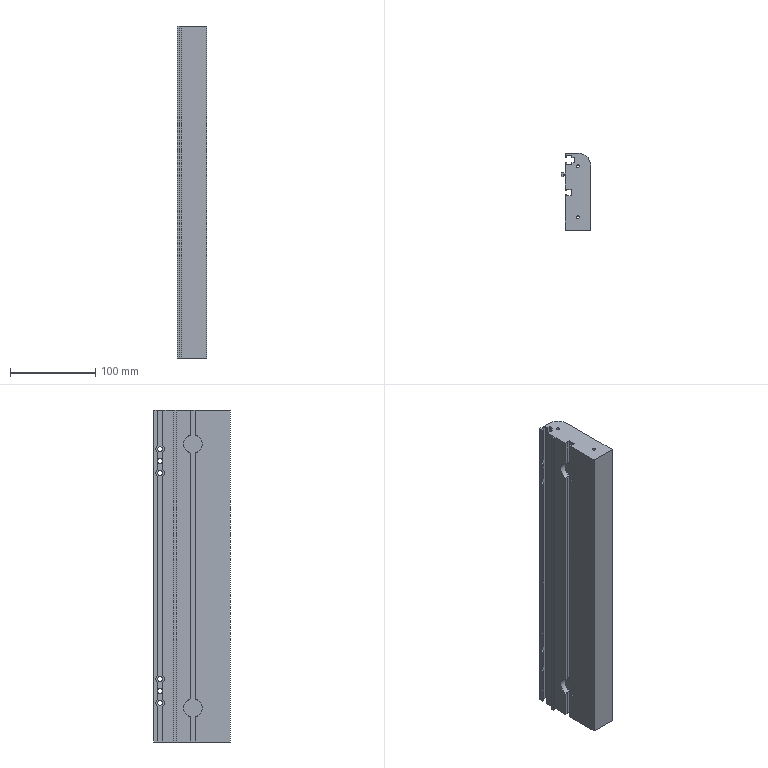Part | SolidWorks | features ICE 3, HoleWzd 2, MirrorPattern 2, Extrusion 1 | 1 solid | 115 faces | box 34.5 x 90 x 390 mm | volume 934909 mm3 | plane 68 | cylinder 47 | commonest cylinder face diameters 10 x16 3.3 x8 5.5 x8 6 x4 20 x4 22 x4